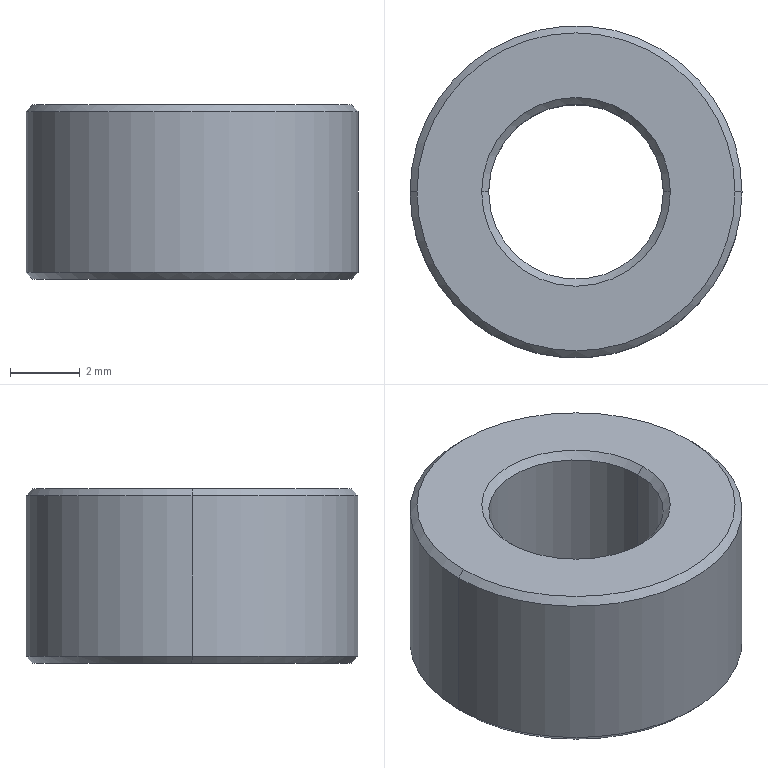Part | STEP file | 1 solid | 14 faces | box 9.5 x 9.5 x 5 mm | volume 254.414 mm3 | cone 8 | cylinder 4 | plane 2 | commonest cylinder face diameters 5 x2 9.5 x2
STEP:
#1=CARTESIAN_POINT('',(0.,0.,0.));
#2=DIRECTION('',(0.,0.,1.));
#3=DIRECTION('',(1.,0.,0.));
#4=AXIS2_PLACEMENT_3D('',#1,#2,#3);
#5=CARTESIAN_POINT('',(-4.55,0.,0.));
#6=VERTEX_POINT('',#5);
#7=CARTESIAN_POINT('',(4.55,0.,0.));
#8=VERTEX_POINT('',#7);
#9=CARTESIAN_POINT('',(0.,0.,0.));
#10=DIRECTION('',(0.,0.,-1.));
#11=DIRECTION('',(1.,0.,0.));
#12=AXIS2_PLACEMENT_3D('',#9,#10,#11);
#13=CIRCLE('',#12,4.55);
#14=CARTESIAN_POINT('',(0.,0.,0.2));
#15=DIRECTION('',(0.,0.,1.));
#16=DIRECTION('',(1.,0.,0.));
#17=AXIS2_PLACEMENT_3D('',#14,#15,#16);
#18=CONICAL_SURFACE('',#17,4.75,0.7854);
#19=CARTESIAN_POINT('',(6.283,-0.2));
#20=DIRECTION('',(-1.,0.));
#21=VECTOR('',#20,1.);
#22=LINE('',#19,#21);
#23=(GEOMETRIC_REPRESENTATION_CONTEXT(2)PARAMETRIC_REPRESENTATION_CONTEXT()REPRESENTATION_CONTEXT('',''));
#24=DEFINITIONAL_REPRESENTATION('',(#22),#23);
#25=PCURVE('',#18,#24);
#26=CARTESIAN_POINT('',(0.,0.,0.));
#27=DIRECTION('',(0.,0.,1.));
#28=DIRECTION('',(1.,0.,0.));
#29=AXIS2_PLACEMENT_3D('',#26,#27,#28);
#30=PLANE('',#29);
#31=CARTESIAN_POINT('',(4.55,0.));
#32=CARTESIAN_POINT('',(4.55,-7.881));
#33=CARTESIAN_POINT('',(-2.275,-3.94));
#34=CARTESIAN_POINT('',(-9.1,0.));
#35=CARTESIAN_POINT('',(-2.275,3.94));
#36=CARTESIAN_POINT('',(4.55,7.881));
#37=CARTESIAN_POINT('',(4.55,0.));
#38=(BOUNDED_CURVE()B_SPLINE_CURVE(2,(#31,#32,#33,#34,#35,#36,#37),.UNSPECIFIED.,.T.,.F.)B_SPLINE_CURVE_WITH_KNOTS((1,2,2,2,2,1),(-2.094,0.,2.094,4.189,6.283,8.378),.UNSPECIFIED.)CURVE()GEOMETRIC_REPRESENTATION_ITEM()RATIONAL_B_SPLINE_CURVE((1.,0.5,1.,0.5,1.,0.5,1.))REPRESENTATION_ITEM(''));
#39=(GEOMETRIC_REPRESENTATION_CONTEXT(2)PARAMETRIC_REPRESENTATION_CONTEXT()REPRESENTATION_CONTEXT('',''));
#40=DEFINITIONAL_REPRESENTATION('',(#38),#39);
#41=PCURVE('',#30,#40);
#42=SURFACE_CURVE('',#13,(#25,#41),.PCURVE_S1.);
#43=EDGE_CURVE('',#6,#8,#42,.T.);
#44=ORIENTED_EDGE('',*,*,#43,.F.);
#45=CARTESIAN_POINT('',(-4.75,0.,0.2));
#46=VERTEX_POINT('',#45);
#47=CARTESIAN_POINT('',(-4.75,0.,0.2));
#48=DIRECTION('',(-0.7071,0.,0.7071));
#49=VECTOR('',#48,1.);
#50=LINE('',#47,#49);
#51=CARTESIAN_POINT('',(3.142,0.));
#52=DIRECTION('',(0.,1.));
#53=VECTOR('',#52,1.);
#54=LINE('',#51,#53);
#55=(GEOMETRIC_REPRESENTATION_CONTEXT(2)PARAMETRIC_REPRESENTATION_CONTEXT()REPRESENTATION_CONTEXT('',''));
#56=DEFINITIONAL_REPRESENTATION('',(#54),#55);
#57=PCURVE('',#18,#56);
#58=CARTESIAN_POINT('',(0.,0.,0.2));
#59=DIRECTION('',(0.,0.,1.));
#60=DIRECTION('',(1.,0.,0.));
#61=AXIS2_PLACEMENT_3D('',#58,#59,#60);
#62=CONICAL_SURFACE('',#61,4.75,0.7854);
#63=CARTESIAN_POINT('',(3.142,0.));
#64=DIRECTION('',(0.,1.));
#65=VECTOR('',#64,1.);
#66=LINE('',#63,#65);
#67=(GEOMETRIC_REPRESENTATION_CONTEXT(2)PARAMETRIC_REPRESENTATION_CONTEXT()REPRESENTATION_CONTEXT('',''));
#68=DEFINITIONAL_REPRESENTATION('',(#66),#67);
#69=PCURVE('',#62,#68);
#70=SURFACE_CURVE('',#50,(#57,#69),.PCURVE_S1.);
#71=EDGE_CURVE('',#6,#46,#70,.T.);
#72=ORIENTED_EDGE('',*,*,#71,.T.);
#73=CARTESIAN_POINT('',(4.75,0.,0.2));
#74=VERTEX_POINT('',#73);
#75=CARTESIAN_POINT('',(0.,0.,0.2));
#76=DIRECTION('',(0.,0.,1.));
#77=DIRECTION('',(1.,0.,0.));
#78=AXIS2_PLACEMENT_3D('',#75,#76,#77);
#79=CIRCLE('',#78,4.75);
#80=CARTESIAN_POINT('',(0.,0.));
#81=DIRECTION('',(1.,0.));
#82=VECTOR('',#81,1.);
#83=LINE('',#80,#82);
#84=(GEOMETRIC_REPRESENTATION_CONTEXT(2)PARAMETRIC_REPRESENTATION_CONTEXT()REPRESENTATION_CONTEXT('',''));
#85=DEFINITIONAL_REPRESENTATION('',(#83),#84);
#86=PCURVE('',#18,#85);
#87=CARTESIAN_POINT('',(0.,0.,5.));
#88=DIRECTION('',(0.,0.,-1.));
#89=DIRECTION('',(-1.,0.,0.));
#90=AXIS2_PLACEMENT_3D('',#87,#88,#89);
#91=CYLINDRICAL_SURFACE('',#90,4.75);
#92=CARTESIAN_POINT('',(3.142,4.8));
#93=DIRECTION('',(-1.,0.));
#94=VECTOR('',#93,1.);
#95=LINE('',#92,#94);
#96=(GEOMETRIC_REPRESENTATION_CONTEXT(2)PARAMETRIC_REPRESENTATION_CONTEXT()REPRESENTATION_CONTEXT('',''));
#97=DEFINITIONAL_REPRESENTATION('',(#95),#96);
#98=PCURVE('',#91,#97);
#99=SURFACE_CURVE('',#79,(#86,#98),.PCURVE_S1.);
#100=EDGE_CURVE('',#74,#46,#99,.T.);
#101=ORIENTED_EDGE('',*,*,#100,.F.);
#102=CARTESIAN_POINT('',(4.75,0.,0.2));
#103=DIRECTION('',(0.7071,0.,0.7071));
#104=VECTOR('',#103,1.);
#105=LINE('',#102,#104);
#106=CARTESIAN_POINT('',(0.,0.));
#107=DIRECTION('',(0.,1.));
#108=VECTOR('',#107,1.);
#109=LINE('',#106,#108);
#110=(GEOMETRIC_REPRESENTATION_CONTEXT(2)PARAMETRIC_REPRESENTATION_CONTEXT()REPRESENTATION_CONTEXT('',''));
#111=DEFINITIONAL_REPRESENTATION('',(#109),#110);
#112=PCURVE('',#18,#111);
#113=CARTESIAN_POINT('',(6.283,0.));
#114=DIRECTION('',(0.,1.));
#115=VECTOR('',#114,1.);
#116=LINE('',#113,#115);
#117=(GEOMETRIC_REPRESENTATION_CONTEXT(2)PARAMETRIC_REPRESENTATION_CONTEXT()REPRESENTATION_CONTEXT('',''));
#118=DEFINITIONAL_REPRESENTATION('',(#116),#117);
#119=PCURVE('',#62,#118);
#120=SURFACE_CURVE('',#105,(#112,#119),.PCURVE_S1.);
#121=EDGE_CURVE('',#8,#74,#120,.T.);
#122=ORIENTED_EDGE('',*,*,#121,.F.);
#123=EDGE_LOOP('',(#44,#72,#101,#122));
#124=FACE_BOUND('',#123,.T.);
#125=ADVANCED_FACE('',(#124),#18,.T.);
#126=CARTESIAN_POINT('',(4.55,0.,5.));
#127=VERTEX_POINT('',#126);
#128=CARTESIAN_POINT('',(-4.55,0.,5.));
#129=VERTEX_POINT('',#128);
#130=CARTESIAN_POINT('',(0.,0.,5.));
#131=DIRECTION('',(0.,0.,1.));
#132=DIRECTION('',(1.,0.,0.));
#133=AXIS2_PLACEMENT_3D('',#130,#131,#132);
#134=CIRCLE('',#133,4.55);
#135=CARTESIAN_POINT('',(0.,0.,5.));
#136=DIRECTION('',(0.,0.,-1.));
#137=DIRECTION('',(-1.,0.,0.));
#138=AXIS2_PLACEMENT_3D('',#135,#136,#137);
#139=CONICAL_SURFACE('',#138,4.55,0.7854);
#140=CARTESIAN_POINT('',(3.142,0.));
#141=DIRECTION('',(-1.,0.));
#142=VECTOR('',#141,1.);
#143=LINE('',#140,#142);
#144=(GEOMETRIC_REPRESENTATION_CONTEXT(2)PARAMETRIC_REPRESENTATION_CONTEXT()REPRESENTATION_CONTEXT('',''));
#145=DEFINITIONAL_REPRESENTATION('',(#143),#144);
#146=PCURVE('',#139,#145);
#147=CARTESIAN_POINT('',(0.,0.,5.));
#148=DIRECTION('',(0.,0.,1.));
#149=DIRECTION('',(1.,0.,0.));
#150=AXIS2_PLACEMENT_3D('',#147,#148,#149);
#151=PLANE('',#150);
#152=CARTESIAN_POINT('',(0.,0.));
#153=DIRECTION('',(1.,0.));
#154=AXIS2_PLACEMENT_2D('',#152,#153);
#155=CIRCLE('',#154,4.55);
#156=(GEOMETRIC_REPRESENTATION_CONTEXT(2)PARAMETRIC_REPRESENTATION_CONTEXT()REPRESENTATION_CONTEXT('',''));
#157=DEFINITIONAL_REPRESENTATION('',(#155),#156);
#158=PCURVE('',#151,#157);
#159=SURFACE_CURVE('',#134,(#146,#158),.PCURVE_S1.);
#160=EDGE_CURVE('',#127,#129,#159,.T.);
#161=ORIENTED_EDGE('',*,*,#160,.F.);
#162=CARTESIAN_POINT('',(4.75,0.,4.8));
#163=VERTEX_POINT('',#162);
#164=CARTESIAN_POINT('',(4.55,0.,5.));
#165=DIRECTION('',(0.7071,0.,-0.7071));
#166=VECTOR('',#165,1.);
#167=LINE('',#164,#166);
#168=CARTESIAN_POINT('',(3.142,0.));
#169=DIRECTION('',(0.,1.));
#170=VECTOR('',#169,1.);
#171=LINE('',#168,#170);
#172=(GEOMETRIC_REPRESENTATION_CONTEXT(2)PARAMETRIC_REPRESENTATION_CONTEXT()REPRESENTATION_CONTEXT('',''));
#173=DEFINITIONAL_REPRESENTATION('',(#171),#172);
#174=PCURVE('',#139,#173);
#175=CARTESIAN_POINT('',(0.,0.,5.));
#176=DIRECTION('',(0.,0.,-1.));
#177=DIRECTION('',(-1.,0.,0.));
#178=AXIS2_PLACEMENT_3D('',#175,#176,#177);
#179=CONICAL_SURFACE('',#178,4.55,0.7854);
#180=CARTESIAN_POINT('',(3.142,0.));
#181=DIRECTION('',(0.,1.));
#182=VECTOR('',#181,1.);
#183=LINE('',#180,#182);
#184=(GEOMETRIC_REPRESENTATION_CONTEXT(2)PARAMETRIC_REPRESENTATION_CONTEXT()REPRESENTATION_CONTEXT('',''));
#185=DEFINITIONAL_REPRESENTATION('',(#183),#184);
#186=PCURVE('',#179,#185);
#187=SURFACE_CURVE('',#167,(#174,#186),.PCURVE_S1.);
#188=EDGE_CURVE('',#127,#163,#187,.T.);
#189=ORIENTED_EDGE('',*,*,#188,.T.);
#190=CARTESIAN_POINT('',(-4.75,0.,4.8));
#191=VERTEX_POINT('',#190);
#192=CARTESIAN_POINT('',(0.,0.,4.8));
#193=DIRECTION('',(0.,0.,-1.));
#194=DIRECTION('',(1.,0.,0.));
#195=AXIS2_PLACEMENT_3D('',#192,#193,#194);
#196=CIRCLE('',#195,4.75);
#197=CARTESIAN_POINT('',(-3.142,0.2));
#198=DIRECTION('',(1.,0.));
#199=VECTOR('',#198,1.);
#200=LINE('',#197,#199);
#201=(GEOMETRIC_REPRESENTATION_CONTEXT(2)PARAMETRIC_REPRESENTATION_CONTEXT()REPRESENTATION_CONTEXT('',''));
#202=DEFINITIONAL_REPRESENTATION('',(#200),#201);
#203=PCURVE('',#139,#202);
#204=CARTESIAN_POINT('',(-3.142,0.2));
#205=DIRECTION('',(1.,0.));
#206=VECTOR('',#205,1.);
#207=LINE('',#204,#206);
#208=(GEOMETRIC_REPRESENTATION_CONTEXT(2)PARAMETRIC_REPRESENTATION_CONTEXT()REPRESENTATION_CONTEXT('',''));
#209=DEFINITIONAL_REPRESENTATION('',(#207),#208);
#210=PCURVE('',#91,#209);
#211=SURFACE_CURVE('',#196,(#203,#210),.PCURVE_S1.);
#212=EDGE_CURVE('',#191,#163,#211,.T.);
#213=ORIENTED_EDGE('',*,*,#212,.F.);
#214=CARTESIAN_POINT('',(-4.55,0.,5.));
#215=DIRECTION('',(-0.7071,0.,-0.7071));
#216=VECTOR('',#215,1.);
#217=LINE('',#214,#216);
#218=CARTESIAN_POINT('',(0.,0.));
#219=DIRECTION('',(0.,1.));
#220=VECTOR('',#219,1.);
#221=LINE('',#218,#220);
#222=(GEOMETRIC_REPRESENTATION_CONTEXT(2)PARAMETRIC_REPRESENTATION_CONTEXT()REPRESENTATION_CONTEXT('',''));
#223=DEFINITIONAL_REPRESENTATION('',(#221),#222);
#224=PCURVE('',#139,#223);
#225=CARTESIAN_POINT('',(6.283,0.));
#226=DIRECTION('',(0.,1.));
#227=VECTOR('',#226,1.);
#228=LINE('',#225,#227);
#229=(GEOMETRIC_REPRESENTATION_CONTEXT(2)PARAMETRIC_REPRESENTATION_CONTEXT()REPRESENTATION_CONTEXT('',''));
#230=DEFINITIONAL_REPRESENTATION('',(#228),#229);
#231=PCURVE('',#179,#230);
#232=SURFACE_CURVE('',#217,(#224,#231),.PCURVE_S1.);
#233=EDGE_CURVE('',#129,#191,#232,.T.);
#234=ORIENTED_EDGE('',*,*,#233,.F.);
#235=EDGE_LOOP('',(#161,#189,#213,#234));
#236=FACE_BOUND('',#235,.T.);
#237=ADVANCED_FACE('',(#236),#139,.T.);
#238=CARTESIAN_POINT('',(2.5,0.,4.8));
#239=VERTEX_POINT('',#238);
#240=CARTESIAN_POINT('',(2.7,0.,5.));
#241=VERTEX_POINT('',#240);
#242=CARTESIAN_POINT('',(2.7,0.,5.));
#243=DIRECTION('',(0.7071,0.,0.7071));
#244=VECTOR('',#243,1.);
#245=LINE('',#242,#244);
#246=CARTESIAN_POINT('',(0.,0.,5.));
#247=DIRECTION('',(0.,0.,1.));
#248=DIRECTION('',(1.,0.,0.));
#249=AXIS2_PLACEMENT_3D('',#246,#247,#248);
#250=CONICAL_SURFACE('',#249,2.7,0.7854);
#251=CARTESIAN_POINT('',(6.283,0.));
#252=DIRECTION('',(0.,1.));
#253=VECTOR('',#252,1.);
#254=LINE('',#251,#253);
#255=(GEOMETRIC_REPRESENTATION_CONTEXT(2)PARAMETRIC_REPRESENTATION_CONTEXT()REPRESENTATION_CONTEXT('',''));
#256=DEFINITIONAL_REPRESENTATION('',(#254),#255);
#257=PCURVE('',#250,#256);
#258=CARTESIAN_POINT('',(0.,0.,5.));
#259=DIRECTION('',(0.,0.,1.));
#260=DIRECTION('',(1.,0.,0.));
#261=AXIS2_PLACEMENT_3D('',#258,#259,#260);
#262=CONICAL_SURFACE('',#261,2.7,0.7854);
#263=CARTESIAN_POINT('',(0.,0.));
#264=DIRECTION('',(0.,1.));
#265=VECTOR('',#264,1.);
#266=LINE('',#263,#265);
#267=(GEOMETRIC_REPRESENTATION_CONTEXT(2)PARAMETRIC_REPRESENTATION_CONTEXT()REPRESENTATION_CONTEXT('',''));
#268=DEFINITIONAL_REPRESENTATION('',(#266),#267);
#269=PCURVE('',#262,#268);
#270=SURFACE_CURVE('',#245,(#257,#269),.PCURVE_S1.);
#271=EDGE_CURVE('',#239,#241,#270,.T.);
#272=ORIENTED_EDGE('',*,*,#271,.T.);
#273=CARTESIAN_POINT('',(-2.7,0.,5.));
#274=VERTEX_POINT('',#273);
#275=CARTESIAN_POINT('',(0.,0.,5.));
#276=DIRECTION('',(0.,0.,-1.));
#277=DIRECTION('',(1.,0.,0.));
#278=AXIS2_PLACEMENT_3D('',#275,#276,#277);
#279=CIRCLE('',#278,2.7);
#280=CARTESIAN_POINT('',(6.283,0.));
#281=DIRECTION('',(-1.,0.));
#282=VECTOR('',#281,1.);
#283=LINE('',#280,#282);
#284=(GEOMETRIC_REPRESENTATION_CONTEXT(2)PARAMETRIC_REPRESENTATION_CONTEXT()REPRESENTATION_CONTEXT('',''));
#285=DEFINITIONAL_REPRESENTATION('',(#283),#284);
#286=PCURVE('',#250,#285);
#287=CARTESIAN_POINT('',(2.7,0.));
#288=CARTESIAN_POINT('',(2.7,-4.677));
#289=CARTESIAN_POINT('',(-1.35,-2.338));
#290=CARTESIAN_POINT('',(-5.4,0.));
#291=CARTESIAN_POINT('',(-1.35,2.338));
#292=CARTESIAN_POINT('',(2.7,4.677));
#293=CARTESIAN_POINT('',(2.7,0.));
#294=(BOUNDED_CURVE()B_SPLINE_CURVE(2,(#287,#288,#289,#290,#291,#292,#293),.UNSPECIFIED.,.T.,.F.)B_SPLINE_CURVE_WITH_KNOTS((1,2,2,2,2,1),(-2.094,0.,2.094,4.189,6.283,8.378),.UNSPECIFIED.)CURVE()GEOMETRIC_REPRESENTATION_ITEM()RATIONAL_B_SPLINE_CURVE((1.,0.5,1.,0.5,1.,0.5,1.))REPRESENTATION_ITEM(''));
#295=(GEOMETRIC_REPRESENTATION_CONTEXT(2)PARAMETRIC_REPRESENTATION_CONTEXT()REPRESENTATION_CONTEXT('',''));
#296=DEFINITIONAL_REPRESENTATION('',(#294),#295);
#297=PCURVE('',#151,#296);
#298=SURFACE_CURVE('',#279,(#286,#297),.PCURVE_S1.);
#299=EDGE_CURVE('',#241,#274,#298,.T.);
#300=ORIENTED_EDGE('',*,*,#299,.T.);
#301=CARTESIAN_POINT('',(-2.5,0.,4.8));
#302=VERTEX_POINT('',#301);
#303=CARTESIAN_POINT('',(-2.7,0.,5.));
#304=DIRECTION('',(-0.7071,0.,0.7071));
#305=VECTOR('',#304,1.);
#306=LINE('',#303,#305);
#307=CARTESIAN_POINT('',(3.142,0.));
#308=DIRECTION('',(0.,1.));
#309=VECTOR('',#308,1.);
#310=LINE('',#307,#309);
#311=(GEOMETRIC_REPRESENTATION_CONTEXT(2)PARAMETRIC_REPRESENTATION_CONTEXT()REPRESENTATION_CONTEXT('',''));
#312=DEFINITIONAL_REPRESENTATION('',(#310),#311);
#313=PCURVE('',#250,#312);
#314=CARTESIAN_POINT('',(3.142,0.));
#315=DIRECTION('',(0.,1.));
#316=VECTOR('',#315,1.);
#317=LINE('',#314,#316);
#318=(GEOMETRIC_REPRESENTATION_CONTEXT(2)PARAMETRIC_REPRESENTATION_CONTEXT()REPRESENTATION_CONTEXT('',''));
#319=DEFINITIONAL_REPRESENTATION('',(#317),#318);
#320=PCURVE('',#262,#319);
#321=SURFACE_CURVE('',#306,(#313,#320),.PCURVE_S1.);
#322=EDGE_CURVE('',#302,#274,#321,.T.);
#323=ORIENTED_EDGE('',*,*,#322,.F.);
#324=CARTESIAN_POINT('',(0.,0.,4.8));
#325=DIRECTION('',(0.,0.,1.));
#326=DIRECTION('',(1.,0.,0.));
#327=AXIS2_PLACEMENT_3D('',#324,#325,#326);
#328=CIRCLE('',#327,2.5);
#329=CARTESIAN_POINT('',(0.,-0.2));
#330=DIRECTION('',(1.,0.));
#331=VECTOR('',#330,1.);
#332=LINE('',#329,#331);
#333=(GEOMETRIC_REPRESENTATION_CONTEXT(2)PARAMETRIC_REPRESENTATION_CONTEXT()REPRESENTATION_CONTEXT('',''));
#334=DEFINITIONAL_REPRESENTATION('',(#332),#333);
#335=PCURVE('',#250,#334);
#336=CARTESIAN_POINT('',(0.,0.,5.));
#337=DIRECTION('',(0.,0.,-1.));
#338=DIRECTION('',(-1.,0.,0.));
#339=AXIS2_PLACEMENT_3D('',#336,#337,#338);
#340=CYLINDRICAL_SURFACE('',#339,2.5);
#341=CARTESIAN_POINT('',(9.425,0.2));
#342=DIRECTION('',(-1.,0.));
#343=VECTOR('',#342,1.);
#344=LINE('',#341,#343);
#345=(GEOMETRIC_REPRESENTATION_CONTEXT(2)PARAMETRIC_REPRESENTATION_CONTEXT()REPRESENTATION_CONTEXT('',''));
#346=DEFINITIONAL_REPRESENTATION('',(#344),#345);
#347=PCURVE('',#340,#346);
#348=SURFACE_CURVE('',#328,(#335,#347),.PCURVE_S1.);
#349=EDGE_CURVE('',#302,#239,#348,.T.);
#350=ORIENTED_EDGE('',*,*,#349,.T.);
#351=EDGE_LOOP('',(#272,#300,#323,#350));
#352=FACE_BOUND('',#351,.F.);
#353=ADVANCED_FACE('',(#352),#250,.F.);
#354=CARTESIAN_POINT('',(-2.5,0.,0.2));
#355=VERTEX_POINT('',#354);
#356=CARTESIAN_POINT('',(-2.7,0.,0.));
#357=VERTEX_POINT('',#356);
#358=CARTESIAN_POINT('',(-2.5,0.,0.2));
#359=DIRECTION('',(-0.7071,0.,-0.7071));
#360=VECTOR('',#359,1.);
#361=LINE('',#358,#360);
#362=CARTESIAN_POINT('',(0.,0.,0.2));
#363=DIRECTION('',(0.,0.,-1.));
#364=DIRECTION('',(-1.,0.,0.));
#365=AXIS2_PLACEMENT_3D('',#362,#363,#364);
#366=CONICAL_SURFACE('',#365,2.5,0.7854);
#367=CARTESIAN_POINT('',(6.283,0.));
#368=DIRECTION('',(0.,1.));
#369=VECTOR('',#368,1.);
#370=LINE('',#367,#369);
#371=(GEOMETRIC_REPRESENTATION_CONTEXT(2)PARAMETRIC_REPRESENTATION_CONTEXT()REPRESENTATION_CONTEXT('',''));
#372=DEFINITIONAL_REPRESENTATION('',(#370),#371);
#373=PCURVE('',#366,#372);
#374=CARTESIAN_POINT('',(0.,0.,0.2));
#375=DIRECTION('',(0.,0.,-1.));
#376=DIRECTION('',(-1.,0.,0.));
#377=AXIS2_PLACEMENT_3D('',#374,#375,#376);
#378=CONICAL_SURFACE('',#377,2.5,0.7854);
#379=CARTESIAN_POINT('',(0.,0.));
#380=DIRECTION('',(0.,1.));
#381=VECTOR('',#380,1.);
#382=LINE('',#379,#381);
#383=(GEOMETRIC_REPRESENTATION_CONTEXT(2)PARAMETRIC_REPRESENTATION_CONTEXT()REPRESENTATION_CONTEXT('',''));
#384=DEFINITIONAL_REPRESENTATION('',(#382),#383);
#385=PCURVE('',#378,#384);
#386=SURFACE_CURVE('',#361,(#373,#385),.PCURVE_S1.);
#387=EDGE_CURVE('',#355,#357,#386,.T.);
#388=ORIENTED_EDGE('',*,*,#387,.T.);
#389=CARTESIAN_POINT('',(2.7,0.,0.));
#390=VERTEX_POINT('',#389);
#391=CARTESIAN_POINT('',(0.,0.,0.));
#392=DIRECTION('',(0.,0.,1.));
#393=DIRECTION('',(1.,0.,0.));
#394=AXIS2_PLACEMENT_3D('',#391,#392,#393);
#395=CIRCLE('',#394,2.7);
#396=CARTESIAN_POINT('',(9.425,0.2));
#397=DIRECTION('',(-1.,0.));
#398=VECTOR('',#397,1.);
#399=LINE('',#396,#398);
#400=(GEOMETRIC_REPRESENTATION_CONTEXT(2)PARAMETRIC_REPRESENTATION_CONTEXT()REPRESENTATION_CONTEXT('',''));
#401=DEFINITIONAL_REPRESENTATION('',(#399),#400);
#402=PCURVE('',#366,#401);
#403=CARTESIAN_POINT('',(0.,0.));
#404=DIRECTION('',(1.,0.));
#405=AXIS2_PLACEMENT_2D('',#403,#404);
#406=CIRCLE('',#405,2.7);
#407=(GEOMETRIC_REPRESENTATION_CONTEXT(2)PARAMETRIC_REPRESENTATION_CONTEXT()REPRESENTATION_CONTEXT('',''));
#408=DEFINITIONAL_REPRESENTATION('',(#406),#407);
#409=PCURVE('',#30,#408);
#410=SURFACE_CURVE('',#395,(#402,#409),.PCURVE_S1.);
#411=EDGE_CURVE('',#357,#390,#410,.T.);
#412=ORIENTED_EDGE('',*,*,#411,.T.);
#413=CARTESIAN_POINT('',(2.5,0.,0.2));
#414=VERTEX_POINT('',#413);
#415=CARTESIAN_POINT('',(2.5,0.,0.2));
#416=DIRECTION('',(0.7071,0.,-0.7071));
#417=VECTOR('',#416,1.);
#418=LINE('',#415,#417);
#419=CARTESIAN_POINT('',(3.142,0.));
#420=DIRECTION('',(0.,1.));
#421=VECTOR('',#420,1.);
#422=LINE('',#419,#421);
#423=(GEOMETRIC_REPRESENTATION_CONTEXT(2)PARAMETRIC_REPRESENTATION_CONTEXT()REPRESENTATION_CONTEXT('',''));
#424=DEFINITIONAL_REPRESENTATION('',(#422),#423);
#425=PCURVE('',#366,#424);
#426=CARTESIAN_POINT('',(3.142,0.));
#427=DIRECTION('',(0.,1.));
#428=VECTOR('',#427,1.);
#429=LINE('',#426,#428);
#430=(GEOMETRIC_REPRESENTATION_CONTEXT(2)PARAMETRIC_REPRESENTATION_CONTEXT()REPRESENTATION_CONTEXT('',''));
#431=DEFINITIONAL_REPRESENTATION('',(#429),#430);
#432=PCURVE('',#378,#431);
#433=SURFACE_CURVE('',#418,(#425,#432),.PCURVE_S1.);
#434=EDGE_CURVE('',#414,#390,#433,.T.);
#435=ORIENTED_EDGE('',*,*,#434,.F.);
#436=CARTESIAN_POINT('',(0.,0.,0.2));
#437=DIRECTION('',(0.,0.,-1.));
#438=DIRECTION('',(1.,0.,0.));
#439=AXIS2_PLACEMENT_3D('',#436,#437,#438);
#440=CIRCLE('',#439,2.5);
#441=CARTESIAN_POINT('',(3.142,0.));
#442=DIRECTION('',(1.,0.));
#443=VECTOR('',#442,1.);
#444=LINE('',#441,#443);
#445=(GEOMETRIC_REPRESENTATION_CONTEXT(2)PARAMETRIC_REPRESENTATION_CONTEXT()REPRESENTATION_CONTEXT('',''));
#446=DEFINITIONAL_REPRESENTATION('',(#444),#445);
#447=PCURVE('',#366,#446);
#448=CARTESIAN_POINT('',(3.142,4.8));
#449=DIRECTION('',(1.,0.));
#450=VECTOR('',#449,1.);
#451=LINE('',#448,#450);
#452=(GEOMETRIC_REPRESENTATION_CONTEXT(2)PARAMETRIC_REPRESENTATION_CONTEXT()REPRESENTATION_CONTEXT('',''));
#453=DEFINITIONAL_REPRESENTATION('',(#451),#452);
#454=PCURVE('',#340,#453);
#455=SURFACE_CURVE('',#440,(#447,#454),.PCURVE_S1.);
#456=EDGE_CURVE('',#414,#355,#455,.T.);
#457=ORIENTED_EDGE('',*,*,#456,.T.);
#458=EDGE_LOOP('',(#388,#412,#435,#457));
#459=FACE_BOUND('',#458,.F.);
#460=ADVANCED_FACE('',(#459),#366,.F.);
#461=CARTESIAN_POINT('',(-2.5,0.,5.));
#462=DIRECTION('',(0.,0.,-1.));
#463=VECTOR('',#462,1.);
#464=LINE('',#461,#463);
#465=CARTESIAN_POINT('',(6.283,0.));
#466=DIRECTION('',(0.,1.));
#467=VECTOR('',#466,1.);
#468=LINE('',#465,#467);
#469=(GEOMETRIC_REPRESENTATION_CONTEXT(2)PARAMETRIC_REPRESENTATION_CONTEXT()REPRESENTATION_CONTEXT('',''));
#470=DEFINITIONAL_REPRESENTATION('',(#468),#469);
#471=PCURVE('',#340,#470);
#472=CARTESIAN_POINT('',(0.,0.,5.));
#473=DIRECTION('',(0.,0.,-1.));
#474=DIRECTION('',(-1.,0.,0.));
#475=AXIS2_PLACEMENT_3D('',#472,#473,#474);
#476=CYLINDRICAL_SURFACE('',#475,2.5);
#477=CARTESIAN_POINT('',(0.,0.));
#478=DIRECTION('',(0.,1.));
#479=VECTOR('',#478,1.);
#480=LINE('',#477,#479);
#481=(GEOMETRIC_REPRESENTATION_CONTEXT(2)PARAMETRIC_REPRESENTATION_CONTEXT()REPRESENTATION_CONTEXT('',''));
#482=DEFINITIONAL_REPRESENTATION('',(#480),#481);
#483=PCURVE('',#476,#482);
#484=SURFACE_CURVE('',#464,(#471,#483),.PCURVE_S1.);
#485=EDGE_CURVE('',#302,#355,#484,.T.);
#486=ORIENTED_EDGE('',*,*,#485,.T.);
#487=ORIENTED_EDGE('',*,*,#456,.F.);
#488=CARTESIAN_POINT('',(2.5,0.,5.));
#489=DIRECTION('',(0.,0.,-1.));
#490=VECTOR('',#489,1.);
#491=LINE('',#488,#490);
#492=CARTESIAN_POINT('',(3.142,0.));
#493=DIRECTION('',(0.,1.));
#494=VECTOR('',#493,1.);
#495=LINE('',#492,#494);
#496=(GEOMETRIC_REPRESENTATION_CONTEXT(2)PARAMETRIC_REPRESENTATION_CONTEXT()REPRESENTATION_CONTEXT('',''));
#497=DEFINITIONAL_REPRESENTATION('',(#495),#496);
#498=PCURVE('',#340,#497);
#499=CARTESIAN_POINT('',(3.142,0.));
#500=DIRECTION('',(0.,1.));
#501=VECTOR('',#500,1.);
#502=LINE('',#499,#501);
#503=(GEOMETRIC_REPRESENTATION_CONTEXT(2)PARAMETRIC_REPRESENTATION_CONTEXT()REPRESENTATION_CONTEXT('',''));
#504=DEFINITIONAL_REPRESENTATION('',(#502),#503);
#505=PCURVE('',#476,#504);
#506=SURFACE_CURVE('',#491,(#498,#505),.PCURVE_S1.);
#507=EDGE_CURVE('',#239,#414,#506,.T.);
#508=ORIENTED_EDGE('',*,*,#507,.F.);
#509=ORIENTED_EDGE('',*,*,#349,.F.);
#510=EDGE_LOOP('',(#486,#487,#508,#509));
#511=FACE_BOUND('',#510,.F.);
#512=ADVANCED_FACE('',(#511),#340,.F.);
#513=ORIENTED_EDGE('',*,*,#212,.T.);
#514=CARTESIAN_POINT('',(4.75,0.,5.));
#515=DIRECTION('',(0.,0.,-1.));
#516=VECTOR('',#515,1.);
#517=LINE('',#514,#516);
#518=CARTESIAN_POINT('',(3.142,0.));
#519=DIRECTION('',(0.,1.));
#520=VECTOR('',#519,1.);
#521=LINE('',#518,#520);
#522=(GEOMETRIC_REPRESENTATION_CONTEXT(2)PARAMETRIC_REPRESENTATION_CONTEXT()REPRESENTATION_CONTEXT('',''));
#523=DEFINITIONAL_REPRESENTATION('',(#521),#522);
#524=PCURVE('',#91,#523);
#525=CARTESIAN_POINT('',(0.,0.,5.));
#526=DIRECTION('',(0.,0.,-1.));
#527=DIRECTION('',(-1.,0.,0.));
#528=AXIS2_PLACEMENT_3D('',#525,#526,#527);
#529=CYLINDRICAL_SURFACE('',#528,4.75);
#530=CARTESIAN_POINT('',(3.142,0.));
#531=DIRECTION('',(0.,1.));
#532=VECTOR('',#531,1.);
#533=LINE('',#530,#532);
#534=(GEOMETRIC_REPRESENTATION_CONTEXT(2)PARAMETRIC_REPRESENTATION_CONTEXT()REPRESENTATION_CONTEXT('',''));
#535=DEFINITIONAL_REPRESENTATION('',(#533),#534);
#536=PCURVE('',#529,#535);
#537=SURFACE_CURVE('',#517,(#524,#536),.PCURVE_S1.);
#538=EDGE_CURVE('',#163,#74,#537,.T.);
#539=ORIENTED_EDGE('',*,*,#538,.T.);
#540=ORIENTED_EDGE('',*,*,#100,.T.);
#541=CARTESIAN_POINT('',(-4.75,0.,5.));
#542=DIRECTION('',(0.,0.,-1.));
#543=VECTOR('',#542,1.);
#544=LINE('',#541,#543);
#545=CARTESIAN_POINT('',(0.,0.));
#546=DIRECTION('',(0.,1.));
#547=VECTOR('',#546,1.);
#548=LINE('',#545,#547);
#549=(GEOMETRIC_REPRESENTATION_CONTEXT(2)PARAMETRIC_REPRESENTATION_CONTEXT()REPRESENTATION_CONTEXT('',''));
#550=DEFINITIONAL_REPRESENTATION('',(#548),#549);
#551=PCURVE('',#91,#550);
#552=CARTESIAN_POINT('',(6.283,0.));
#553=DIRECTION('',(0.,1.));
#554=VECTOR('',#553,1.);
#555=LINE('',#552,#554);
#556=(GEOMETRIC_REPRESENTATION_CONTEXT(2)PARAMETRIC_REPRESENTATION_CONTEXT()REPRESENTATION_CONTEXT('',''));
#557=DEFINITIONAL_REPRESENTATION('',(#555),#556);
#558=PCURVE('',#529,#557);
#559=SURFACE_CURVE('',#544,(#551,#558),.PCURVE_S1.);
#560=EDGE_CURVE('',#191,#46,#559,.T.);
#561=ORIENTED_EDGE('',*,*,#560,.F.);
#562=EDGE_LOOP('',(#513,#539,#540,#561));
#563=FACE_BOUND('',#562,.T.);
#564=ADVANCED_FACE('',(#563),#91,.T.);
#565=ORIENTED_EDGE('',*,*,#538,.F.);
#566=CARTESIAN_POINT('',(0.,0.,4.8));
#567=DIRECTION('',(0.,0.,-1.));
#568=DIRECTION('',(1.,0.,0.));
#569=AXIS2_PLACEMENT_3D('',#566,#567,#568);
#570=CIRCLE('',#569,4.75);
#571=CARTESIAN_POINT('',(3.142,0.2));
#572=DIRECTION('',(1.,0.));
#573=VECTOR('',#572,1.);
#574=LINE('',#571,#573);
#575=(GEOMETRIC_REPRESENTATION_CONTEXT(2)PARAMETRIC_REPRESENTATION_CONTEXT()REPRESENTATION_CONTEXT('',''));
#576=DEFINITIONAL_REPRESENTATION('',(#574),#575);
#577=PCURVE('',#529,#576);
#578=CARTESIAN_POINT('',(3.142,0.2));
#579=DIRECTION('',(1.,0.));
#580=VECTOR('',#579,1.);
#581=LINE('',#578,#580);
#582=(GEOMETRIC_REPRESENTATION_CONTEXT(2)PARAMETRIC_REPRESENTATION_CONTEXT()REPRESENTATION_CONTEXT('',''));
#583=DEFINITIONAL_REPRESENTATION('',(#581),#582);
#584=PCURVE('',#179,#583);
#585=SURFACE_CURVE('',#570,(#577,#584),.PCURVE_S1.);
#586=EDGE_CURVE('',#163,#191,#585,.T.);
#587=ORIENTED_EDGE('',*,*,#586,.T.);
#588=ORIENTED_EDGE('',*,*,#560,.T.);
#589=CARTESIAN_POINT('',(0.,0.,0.2));
#590=DIRECTION('',(0.,0.,1.));
#591=DIRECTION('',(1.,0.,0.));
#592=AXIS2_PLACEMENT_3D('',#589,#590,#591);
#593=CIRCLE('',#592,4.75);
#594=CARTESIAN_POINT('',(9.425,4.8));
#595=DIRECTION('',(-1.,0.));
#596=VECTOR('',#595,1.);
#597=LINE('',#594,#596);
#598=(GEOMETRIC_REPRESENTATION_CONTEXT(2)PARAMETRIC_REPRESENTATION_CONTEXT()REPRESENTATION_CONTEXT('',''));
#599=DEFINITIONAL_REPRESENTATION('',(#597),#598);
#600=PCURVE('',#529,#599);
#601=CARTESIAN_POINT('',(0.,0.));
#602=DIRECTION('',(1.,0.));
#603=VECTOR('',#602,1.);
#604=LINE('',#601,#603);
#605=(GEOMETRIC_REPRESENTATION_CONTEXT(2)PARAMETRIC_REPRESENTATION_CONTEXT()REPRESENTATION_CONTEXT('',''));
#606=DEFINITIONAL_REPRESENTATION('',(#604),#605);
#607=PCURVE('',#62,#606);
#608=SURFACE_CURVE('',#593,(#600,#607),.PCURVE_S1.);
#609=EDGE_CURVE('',#46,#74,#608,.T.);
#610=ORIENTED_EDGE('',*,*,#609,.T.);
#611=EDGE_LOOP('',(#565,#587,#588,#610));
#612=FACE_BOUND('',#611,.T.);
#613=ADVANCED_FACE('',(#612),#529,.T.);
#614=ORIENTED_EDGE('',*,*,#299,.T.);
#615=CARTESIAN_POINT('',(0.,0.,5.));
#616=DIRECTION('',(0.,0.,-1.));
#617=DIRECTION('',(1.,0.,0.));
#618=AXIS2_PLACEMENT_3D('',#615,#616,#617);
#619=CIRCLE('',#618,2.7);
#620=CARTESIAN_POINT('',(2.7,0.));
#621=CARTESIAN_POINT('',(2.7,-4.677));
#622=CARTESIAN_POINT('',(-1.35,-2.338));
#623=CARTESIAN_POINT('',(-5.4,0.));
#624=CARTESIAN_POINT('',(-1.35,2.338));
#625=CARTESIAN_POINT('',(2.7,4.677));
#626=CARTESIAN_POINT('',(2.7,0.));
#627=(BOUNDED_CURVE()B_SPLINE_CURVE(2,(#620,#621,#622,#623,#624,#625,#626),.UNSPECIFIED.,.T.,.F.)B_SPLINE_CURVE_WITH_KNOTS((1,2,2,2,2,1),(-2.094,0.,2.094,4.189,6.283,8.378),.UNSPECIFIED.)CURVE()GEOMETRIC_REPRESENTATION_ITEM()RATIONAL_B_SPLINE_CURVE((1.,0.5,1.,0.5,1.,0.5,1.))REPRESENTATION_ITEM(''));
#628=(GEOMETRIC_REPRESENTATION_CONTEXT(2)PARAMETRIC_REPRESENTATION_CONTEXT()REPRESENTATION_CONTEXT('',''));
#629=DEFINITIONAL_REPRESENTATION('',(#627),#628);
#630=PCURVE('',#151,#629);
#631=CARTESIAN_POINT('',(6.283,0.));
#632=DIRECTION('',(-1.,0.));
#633=VECTOR('',#632,1.);
#634=LINE('',#631,#633);
#635=(GEOMETRIC_REPRESENTATION_CONTEXT(2)PARAMETRIC_REPRESENTATION_CONTEXT()REPRESENTATION_CONTEXT('',''));
#636=DEFINITIONAL_REPRESENTATION('',(#634),#635);
#637=PCURVE('',#262,#636);
#638=SURFACE_CURVE('',#619,(#630,#637),.PCURVE_S1.);
#639=EDGE_CURVE('',#274,#241,#638,.T.);
#640=ORIENTED_EDGE('',*,*,#639,.T.);
#641=EDGE_LOOP('',(#614,#640));
#642=FACE_BOUND('',#641,.T.);
#643=CARTESIAN_POINT('',(0.,0.,5.));
#644=DIRECTION('',(0.,0.,1.));
#645=DIRECTION('',(1.,0.,0.));
#646=AXIS2_PLACEMENT_3D('',#643,#644,#645);
#647=CIRCLE('',#646,4.55);
#648=CARTESIAN_POINT('',(0.,0.));
#649=DIRECTION('',(1.,0.));
#650=AXIS2_PLACEMENT_2D('',#648,#649);
#651=CIRCLE('',#650,4.55);
#652=(GEOMETRIC_REPRESENTATION_CONTEXT(2)PARAMETRIC_REPRESENTATION_CONTEXT()REPRESENTATION_CONTEXT('',''));
#653=DEFINITIONAL_REPRESENTATION('',(#651),#652);
#654=PCURVE('',#151,#653);
#655=CARTESIAN_POINT('',(9.425,0.));
#656=DIRECTION('',(-1.,0.));
#657=VECTOR('',#656,1.);
#658=LINE('',#655,#657);
#659=(GEOMETRIC_REPRESENTATION_CONTEXT(2)PARAMETRIC_REPRESENTATION_CONTEXT()REPRESENTATION_CONTEXT('',''));
#660=DEFINITIONAL_REPRESENTATION('',(#658),#659);
#661=PCURVE('',#179,#660);
#662=SURFACE_CURVE('',#647,(#654,#661),.PCURVE_S1.);
#663=EDGE_CURVE('',#129,#127,#662,.T.);
#664=ORIENTED_EDGE('',*,*,#663,.T.);
#665=ORIENTED_EDGE('',*,*,#160,.T.);
#666=EDGE_LOOP('',(#664,#665));
#667=FACE_BOUND('',#666,.T.);
#668=ADVANCED_FACE('',(#642,#667),#151,.T.);
#669=ORIENTED_EDGE('',*,*,#411,.T.);
#670=CARTESIAN_POINT('',(0.,0.,0.));
#671=DIRECTION('',(0.,0.,1.));
#672=DIRECTION('',(1.,0.,0.));
#673=AXIS2_PLACEMENT_3D('',#670,#671,#672);
#674=CIRCLE('',#673,2.7);
#675=CARTESIAN_POINT('',(0.,0.));
#676=DIRECTION('',(1.,0.));
#677=AXIS2_PLACEMENT_2D('',#675,#676);
#678=CIRCLE('',#677,2.7);
#679=(GEOMETRIC_REPRESENTATION_CONTEXT(2)PARAMETRIC_REPRESENTATION_CONTEXT()REPRESENTATION_CONTEXT('',''));
#680=DEFINITIONAL_REPRESENTATION('',(#678),#679);
#681=PCURVE('',#30,#680);
#682=CARTESIAN_POINT('',(3.142,0.2));
#683=DIRECTION('',(-1.,0.));
#684=VECTOR('',#683,1.);
#685=LINE('',#682,#684);
#686=(GEOMETRIC_REPRESENTATION_CONTEXT(2)PARAMETRIC_REPRESENTATION_CONTEXT()REPRESENTATION_CONTEXT('',''));
#687=DEFINITIONAL_REPRESENTATION('',(#685),#686);
#688=PCURVE('',#378,#687);
#689=SURFACE_CURVE('',#674,(#681,#688),.PCURVE_S1.);
#690=EDGE_CURVE('',#390,#357,#689,.T.);
#691=ORIENTED_EDGE('',*,*,#690,.T.);
#692=EDGE_LOOP('',(#669,#691));
#693=FACE_BOUND('',#692,.T.);
#694=CARTESIAN_POINT('',(0.,0.,0.));
#695=DIRECTION('',(0.,0.,-1.));
#696=DIRECTION('',(1.,0.,0.));
#697=AXIS2_PLACEMENT_3D('',#694,#695,#696);
#698=CIRCLE('',#697,4.55);
#699=CARTESIAN_POINT('',(4.55,0.));
#700=CARTESIAN_POINT('',(4.55,-7.881));
#701=CARTESIAN_POINT('',(-2.275,-3.94));
#702=CARTESIAN_POINT('',(-9.1,0.));
#703=CARTESIAN_POINT('',(-2.275,3.94));
#704=CARTESIAN_POINT('',(4.55,7.881));
#705=CARTESIAN_POINT('',(4.55,0.));
#706=(BOUNDED_CURVE()B_SPLINE_CURVE(2,(#699,#700,#701,#702,#703,#704,#705),.UNSPECIFIED.,.T.,.F.)B_SPLINE_CURVE_WITH_KNOTS((1,2,2,2,2,1),(-2.094,0.,2.094,4.189,6.283,8.378),.UNSPECIFIED.)CURVE()GEOMETRIC_REPRESENTATION_ITEM()RATIONAL_B_SPLINE_CURVE((1.,0.5,1.,0.5,1.,0.5,1.))REPRESENTATION_ITEM(''));
#707=(GEOMETRIC_REPRESENTATION_CONTEXT(2)PARAMETRIC_REPRESENTATION_CONTEXT()REPRESENTATION_CONTEXT('',''));
#708=DEFINITIONAL_REPRESENTATION('',(#706),#707);
#709=PCURVE('',#30,#708);
#710=CARTESIAN_POINT('',(6.283,-0.2));
#711=DIRECTION('',(-1.,0.));
#712=VECTOR('',#711,1.);
#713=LINE('',#710,#712);
#714=(GEOMETRIC_REPRESENTATION_CONTEXT(2)PARAMETRIC_REPRESENTATION_CONTEXT()REPRESENTATION_CONTEXT('',''));
#715=DEFINITIONAL_REPRESENTATION('',(#713),#714);
#716=PCURVE('',#62,#715);
#717=SURFACE_CURVE('',#698,(#709,#716),.PCURVE_S1.);
#718=EDGE_CURVE('',#8,#6,#717,.T.);
#719=ORIENTED_EDGE('',*,*,#718,.T.);
#720=ORIENTED_EDGE('',*,*,#43,.T.);
#721=EDGE_LOOP('',(#719,#720));
#722=FACE_BOUND('',#721,.T.);
#723=ADVANCED_FACE('',(#693,#722),#30,.F.);
#724=CARTESIAN_POINT('',(0.,0.,0.2));
#725=DIRECTION('',(0.,0.,-1.));
#726=DIRECTION('',(1.,0.,0.));
#727=AXIS2_PLACEMENT_3D('',#724,#725,#726);
#728=CIRCLE('',#727,2.5);
#729=CARTESIAN_POINT('',(-3.142,4.8));
#730=DIRECTION('',(1.,0.));
#731=VECTOR('',#730,1.);
#732=LINE('',#729,#731);
#733=(GEOMETRIC_REPRESENTATION_CONTEXT(2)PARAMETRIC_REPRESENTATION_CONTEXT()REPRESENTATION_CONTEXT('',''));
#734=DEFINITIONAL_REPRESENTATION('',(#732),#733);
#735=PCURVE('',#476,#734);
#736=CARTESIAN_POINT('',(-3.142,0.));
#737=DIRECTION('',(1.,0.));
#738=VECTOR('',#737,1.);
#739=LINE('',#736,#738);
#740=(GEOMETRIC_REPRESENTATION_CONTEXT(2)PARAMETRIC_REPRESENTATION_CONTEXT()REPRESENTATION_CONTEXT('',''));
#741=DEFINITIONAL_REPRESENTATION('',(#739),#740);
#742=PCURVE('',#378,#741);
#743=SURFACE_CURVE('',#728,(#735,#742),.PCURVE_S1.);
#744=EDGE_CURVE('',#355,#414,#743,.T.);
#745=ORIENTED_EDGE('',*,*,#744,.F.);
#746=ORIENTED_EDGE('',*,*,#485,.F.);
#747=CARTESIAN_POINT('',(0.,0.,4.8));
#748=DIRECTION('',(0.,0.,1.));
#749=DIRECTION('',(1.,0.,0.));
#750=AXIS2_PLACEMENT_3D('',#747,#748,#749);
#751=CIRCLE('',#750,2.5);
#752=CARTESIAN_POINT('',(3.142,0.2));
#753=DIRECTION('',(-1.,0.));
#754=VECTOR('',#753,1.);
#755=LINE('',#752,#754);
#756=(GEOMETRIC_REPRESENTATION_CONTEXT(2)PARAMETRIC_REPRESENTATION_CONTEXT()REPRESENTATION_CONTEXT('',''));
#757=DEFINITIONAL_REPRESENTATION('',(#755),#756);
#758=PCURVE('',#476,#757);
#759=CARTESIAN_POINT('',(0.,-0.2));
#760=DIRECTION('',(1.,0.));
#761=VECTOR('',#760,1.);
#762=LINE('',#759,#761);
#763=(GEOMETRIC_REPRESENTATION_CONTEXT(2)PARAMETRIC_REPRESENTATION_CONTEXT()REPRESENTATION_CONTEXT('',''));
#764=DEFINITIONAL_REPRESENTATION('',(#762),#763);
#765=PCURVE('',#262,#764);
#766=SURFACE_CURVE('',#751,(#758,#765),.PCURVE_S1.);
#767=EDGE_CURVE('',#239,#302,#766,.T.);
#768=ORIENTED_EDGE('',*,*,#767,.F.);
#769=ORIENTED_EDGE('',*,*,#507,.T.);
#770=EDGE_LOOP('',(#745,#746,#768,#769));
#771=FACE_BOUND('',#770,.F.);
#772=ADVANCED_FACE('',(#771),#476,.F.);
#773=ORIENTED_EDGE('',*,*,#690,.T.);
#774=ORIENTED_EDGE('',*,*,#387,.F.);
#775=ORIENTED_EDGE('',*,*,#744,.T.);
#776=ORIENTED_EDGE('',*,*,#434,.T.);
#777=EDGE_LOOP('',(#773,#774,#775,#776));
#778=FACE_BOUND('',#777,.F.);
#779=ADVANCED_FACE('',(#778),#378,.F.);
#780=ORIENTED_EDGE('',*,*,#639,.T.);
#781=ORIENTED_EDGE('',*,*,#271,.F.);
#782=ORIENTED_EDGE('',*,*,#767,.T.);
#783=ORIENTED_EDGE('',*,*,#322,.T.);
#784=EDGE_LOOP('',(#780,#781,#782,#783));
#785=FACE_BOUND('',#784,.F.);
#786=ADVANCED_FACE('',(#785),#262,.F.);
#787=ORIENTED_EDGE('',*,*,#188,.F.);
#788=ORIENTED_EDGE('',*,*,#663,.F.);
#789=ORIENTED_EDGE('',*,*,#233,.T.);
#790=ORIENTED_EDGE('',*,*,#586,.F.);
#791=EDGE_LOOP('',(#787,#788,#789,#790));
#792=FACE_BOUND('',#791,.T.);
#793=ADVANCED_FACE('',(#792),#179,.T.);
#794=ORIENTED_EDGE('',*,*,#71,.F.);
#795=ORIENTED_EDGE('',*,*,#718,.F.);
#796=ORIENTED_EDGE('',*,*,#121,.T.);
#797=ORIENTED_EDGE('',*,*,#609,.F.);
#798=EDGE_LOOP('',(#794,#795,#796,#797));
#799=FACE_BOUND('',#798,.T.);
#800=ADVANCED_FACE('',(#799),#62,.T.);
#801=CLOSED_SHELL('',(#125,#237,#353,#460,#512,#564,#613,#668,#723,#772,#779,#786,#793,#800));
#802=MANIFOLD_SOLID_BREP('',#801);
#803=(LENGTH_UNIT()NAMED_UNIT(*)SI_UNIT(.MILLI.,.METRE.));
#804=UNCERTAINTY_MEASURE_WITH_UNIT(LENGTH_MEASURE(0.0000001),#803,'','');
#805=(NAMED_UNIT(*)PLANE_ANGLE_UNIT()SI_UNIT($,.RADIAN.));
#806=(NAMED_UNIT(*)SI_UNIT($,.STERADIAN.)SOLID_ANGLE_UNIT());
#807=(GEOMETRIC_REPRESENTATION_CONTEXT(3)GLOBAL_UNCERTAINTY_ASSIGNED_CONTEXT((#804))GLOBAL_UNIT_ASSIGNED_CONTEXT((#803,#805,#806))REPRESENTATION_CONTEXT('',''));
#808=ADVANCED_BREP_SHAPE_REPRESENTATION('',(#4,#802),#807);